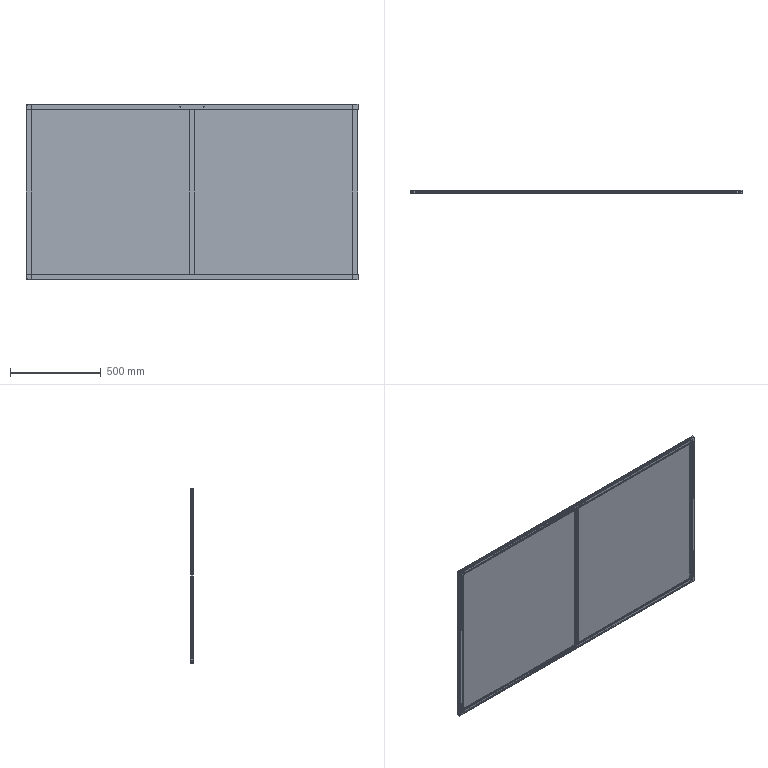Part | SolidWorks | features ReferencePattern 2, LocalLPattern 1 | 21 solids | 989 faces | box 1832 x 15 x 970 mm | volume 9765548 mm3 | plane 600 | cylinder 269 | cone 68 | spline 52 | commonest cylinder face diameters 5 x67 11 x52 1 x42 3.3 x24 2 x20 6 x20